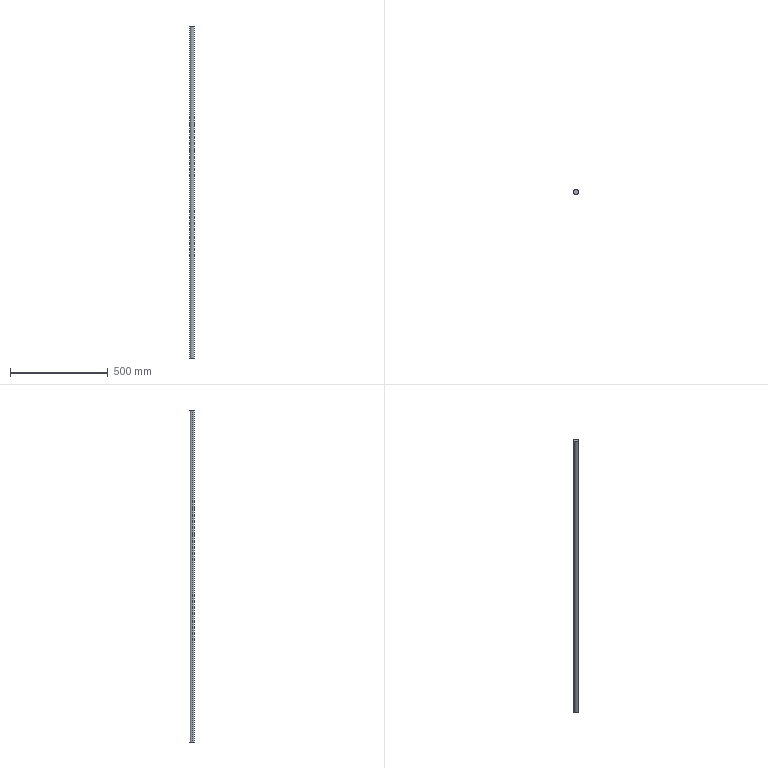Part | STEP file | 管-1700 | 1 solid | 4 faces | box 25.4 x 25.4 x 1700 mm | volume 861403 mm3 | cylinder 2 | plane 2 | commonest cylinder face diameters 25.4 x2
STEP:
#1=CARTESIAN_POINT('',(0.,0.,0.));
#2=DIRECTION('',(0.,0.,1.));
#3=DIRECTION('',(1.,0.,0.));
#4=AXIS2_PLACEMENT_3D('',#1,#2,#3);
#5=CARTESIAN_POINT('',(12.7,0.,850.));
#6=VERTEX_POINT('',#5);
#7=CARTESIAN_POINT('',(-12.7,0.,850.));
#8=VERTEX_POINT('',#7);
#9=CARTESIAN_POINT('',(0.,0.,850.));
#10=DIRECTION('',(0.,0.,1.));
#11=DIRECTION('',(1.,0.,0.));
#12=AXIS2_PLACEMENT_3D('',#9,#10,#11);
#13=CIRCLE('',#12,12.7);
#14=CARTESIAN_POINT('',(0.,0.,850.));
#15=DIRECTION('',(0.,0.,-1.));
#16=DIRECTION('',(-1.,0.,0.));
#17=AXIS2_PLACEMENT_3D('',#14,#15,#16);
#18=CYLINDRICAL_SURFACE('',#17,12.7);
#19=CARTESIAN_POINT('',(3.142,0.));
#20=DIRECTION('',(-1.,0.));
#21=VECTOR('',#20,1.);
#22=LINE('',#19,#21);
#23=(GEOMETRIC_REPRESENTATION_CONTEXT(2)PARAMETRIC_REPRESENTATION_CONTEXT()REPRESENTATION_CONTEXT('',''));
#24=DEFINITIONAL_REPRESENTATION('',(#22),#23);
#25=PCURVE('',#18,#24);
#26=CARTESIAN_POINT('',(0.,0.,850.));
#27=DIRECTION('',(0.,0.,1.));
#28=DIRECTION('',(1.,0.,0.));
#29=AXIS2_PLACEMENT_3D('',#26,#27,#28);
#30=PLANE('',#29);
#31=CARTESIAN_POINT('',(0.,0.));
#32=DIRECTION('',(1.,0.));
#33=AXIS2_PLACEMENT_2D('',#31,#32);
#34=CIRCLE('',#33,12.7);
#35=(GEOMETRIC_REPRESENTATION_CONTEXT(2)PARAMETRIC_REPRESENTATION_CONTEXT()REPRESENTATION_CONTEXT('',''));
#36=DEFINITIONAL_REPRESENTATION('',(#34),#35);
#37=PCURVE('',#30,#36);
#38=SURFACE_CURVE('',#13,(#25,#37),.PCURVE_S1.);
#39=EDGE_CURVE('',#6,#8,#38,.T.);
#40=ORIENTED_EDGE('',*,*,#39,.F.);
#41=CARTESIAN_POINT('',(12.7,0.,-850.));
#42=VERTEX_POINT('',#41);
#43=CARTESIAN_POINT('',(12.7,0.,850.));
#44=DIRECTION('',(0.,0.,-1.));
#45=VECTOR('',#44,1.);
#46=LINE('',#43,#45);
#47=CARTESIAN_POINT('',(3.142,0.));
#48=DIRECTION('',(0.,1.));
#49=VECTOR('',#48,1.);
#50=LINE('',#47,#49);
#51=(GEOMETRIC_REPRESENTATION_CONTEXT(2)PARAMETRIC_REPRESENTATION_CONTEXT()REPRESENTATION_CONTEXT('',''));
#52=DEFINITIONAL_REPRESENTATION('',(#50),#51);
#53=PCURVE('',#18,#52);
#54=CARTESIAN_POINT('',(0.,0.,850.));
#55=DIRECTION('',(0.,0.,-1.));
#56=DIRECTION('',(-1.,0.,0.));
#57=AXIS2_PLACEMENT_3D('',#54,#55,#56);
#58=CYLINDRICAL_SURFACE('',#57,12.7);
#59=CARTESIAN_POINT('',(3.142,0.));
#60=DIRECTION('',(0.,1.));
#61=VECTOR('',#60,1.);
#62=LINE('',#59,#61);
#63=(GEOMETRIC_REPRESENTATION_CONTEXT(2)PARAMETRIC_REPRESENTATION_CONTEXT()REPRESENTATION_CONTEXT('',''));
#64=DEFINITIONAL_REPRESENTATION('',(#62),#63);
#65=PCURVE('',#58,#64);
#66=SURFACE_CURVE('',#46,(#53,#65),.PCURVE_S1.);
#67=EDGE_CURVE('',#6,#42,#66,.T.);
#68=ORIENTED_EDGE('',*,*,#67,.T.);
#69=CARTESIAN_POINT('',(-12.7,0.,-850.));
#70=VERTEX_POINT('',#69);
#71=CARTESIAN_POINT('',(0.,0.,-850.));
#72=DIRECTION('',(0.,0.,1.));
#73=DIRECTION('',(1.,0.,0.));
#74=AXIS2_PLACEMENT_3D('',#71,#72,#73);
#75=CIRCLE('',#74,12.7);
#76=CARTESIAN_POINT('',(3.142,1700.));
#77=DIRECTION('',(-1.,0.));
#78=VECTOR('',#77,1.);
#79=LINE('',#76,#78);
#80=(GEOMETRIC_REPRESENTATION_CONTEXT(2)PARAMETRIC_REPRESENTATION_CONTEXT()REPRESENTATION_CONTEXT('',''));
#81=DEFINITIONAL_REPRESENTATION('',(#79),#80);
#82=PCURVE('',#18,#81);
#83=CARTESIAN_POINT('',(0.,0.,-850.));
#84=DIRECTION('',(0.,0.,1.));
#85=DIRECTION('',(1.,0.,0.));
#86=AXIS2_PLACEMENT_3D('',#83,#84,#85);
#87=PLANE('',#86);
#88=CARTESIAN_POINT('',(0.,0.));
#89=DIRECTION('',(1.,0.));
#90=AXIS2_PLACEMENT_2D('',#88,#89);
#91=CIRCLE('',#90,12.7);
#92=(GEOMETRIC_REPRESENTATION_CONTEXT(2)PARAMETRIC_REPRESENTATION_CONTEXT()REPRESENTATION_CONTEXT('',''));
#93=DEFINITIONAL_REPRESENTATION('',(#91),#92);
#94=PCURVE('',#87,#93);
#95=SURFACE_CURVE('',#75,(#82,#94),.PCURVE_S1.);
#96=EDGE_CURVE('',#42,#70,#95,.T.);
#97=ORIENTED_EDGE('',*,*,#96,.T.);
#98=CARTESIAN_POINT('',(-12.7,0.,850.));
#99=DIRECTION('',(0.,0.,-1.));
#100=VECTOR('',#99,1.);
#101=LINE('',#98,#100);
#102=CARTESIAN_POINT('',(0.,0.));
#103=DIRECTION('',(0.,1.));
#104=VECTOR('',#103,1.);
#105=LINE('',#102,#104);
#106=(GEOMETRIC_REPRESENTATION_CONTEXT(2)PARAMETRIC_REPRESENTATION_CONTEXT()REPRESENTATION_CONTEXT('',''));
#107=DEFINITIONAL_REPRESENTATION('',(#105),#106);
#108=PCURVE('',#18,#107);
#109=CARTESIAN_POINT('',(6.283,0.));
#110=DIRECTION('',(0.,1.));
#111=VECTOR('',#110,1.);
#112=LINE('',#109,#111);
#113=(GEOMETRIC_REPRESENTATION_CONTEXT(2)PARAMETRIC_REPRESENTATION_CONTEXT()REPRESENTATION_CONTEXT('',''));
#114=DEFINITIONAL_REPRESENTATION('',(#112),#113);
#115=PCURVE('',#58,#114);
#116=SURFACE_CURVE('',#101,(#108,#115),.PCURVE_S1.);
#117=EDGE_CURVE('',#8,#70,#116,.T.);
#118=ORIENTED_EDGE('',*,*,#117,.F.);
#119=EDGE_LOOP('',(#40,#68,#97,#118));
#120=FACE_BOUND('',#119,.T.);
#121=ADVANCED_FACE('',(#120),#18,.T.);
#122=ORIENTED_EDGE('',*,*,#67,.F.);
#123=CARTESIAN_POINT('',(0.,0.,850.));
#124=DIRECTION('',(0.,0.,1.));
#125=DIRECTION('',(1.,0.,0.));
#126=AXIS2_PLACEMENT_3D('',#123,#124,#125);
#127=CIRCLE('',#126,12.7);
#128=CARTESIAN_POINT('',(9.425,0.));
#129=DIRECTION('',(-1.,0.));
#130=VECTOR('',#129,1.);
#131=LINE('',#128,#130);
#132=(GEOMETRIC_REPRESENTATION_CONTEXT(2)PARAMETRIC_REPRESENTATION_CONTEXT()REPRESENTATION_CONTEXT('',''));
#133=DEFINITIONAL_REPRESENTATION('',(#131),#132);
#134=PCURVE('',#58,#133);
#135=CARTESIAN_POINT('',(0.,0.));
#136=DIRECTION('',(1.,0.));
#137=AXIS2_PLACEMENT_2D('',#135,#136);
#138=CIRCLE('',#137,12.7);
#139=(GEOMETRIC_REPRESENTATION_CONTEXT(2)PARAMETRIC_REPRESENTATION_CONTEXT()REPRESENTATION_CONTEXT('',''));
#140=DEFINITIONAL_REPRESENTATION('',(#138),#139);
#141=PCURVE('',#30,#140);
#142=SURFACE_CURVE('',#127,(#134,#141),.PCURVE_S1.);
#143=EDGE_CURVE('',#8,#6,#142,.T.);
#144=ORIENTED_EDGE('',*,*,#143,.F.);
#145=ORIENTED_EDGE('',*,*,#117,.T.);
#146=CARTESIAN_POINT('',(0.,0.,-850.));
#147=DIRECTION('',(0.,0.,1.));
#148=DIRECTION('',(1.,0.,0.));
#149=AXIS2_PLACEMENT_3D('',#146,#147,#148);
#150=CIRCLE('',#149,12.7);
#151=CARTESIAN_POINT('',(9.425,1700.));
#152=DIRECTION('',(-1.,0.));
#153=VECTOR('',#152,1.);
#154=LINE('',#151,#153);
#155=(GEOMETRIC_REPRESENTATION_CONTEXT(2)PARAMETRIC_REPRESENTATION_CONTEXT()REPRESENTATION_CONTEXT('',''));
#156=DEFINITIONAL_REPRESENTATION('',(#154),#155);
#157=PCURVE('',#58,#156);
#158=CARTESIAN_POINT('',(0.,0.));
#159=DIRECTION('',(1.,0.));
#160=AXIS2_PLACEMENT_2D('',#158,#159);
#161=CIRCLE('',#160,12.7);
#162=(GEOMETRIC_REPRESENTATION_CONTEXT(2)PARAMETRIC_REPRESENTATION_CONTEXT()REPRESENTATION_CONTEXT('',''));
#163=DEFINITIONAL_REPRESENTATION('',(#161),#162);
#164=PCURVE('',#87,#163);
#165=SURFACE_CURVE('',#150,(#157,#164),.PCURVE_S1.);
#166=EDGE_CURVE('',#70,#42,#165,.T.);
#167=ORIENTED_EDGE('',*,*,#166,.T.);
#168=EDGE_LOOP('',(#122,#144,#145,#167));
#169=FACE_BOUND('',#168,.T.);
#170=ADVANCED_FACE('',(#169),#58,.T.);
#171=ORIENTED_EDGE('',*,*,#143,.T.);
#172=ORIENTED_EDGE('',*,*,#39,.T.);
#173=EDGE_LOOP('',(#171,#172));
#174=FACE_BOUND('',#173,.T.);
#175=ADVANCED_FACE('',(#174),#30,.T.);
#176=ORIENTED_EDGE('',*,*,#166,.F.);
#177=ORIENTED_EDGE('',*,*,#96,.F.);
#178=EDGE_LOOP('',(#176,#177));
#179=FACE_BOUND('',#178,.T.);
#180=ADVANCED_FACE('',(#179),#87,.F.);
#181=CLOSED_SHELL('',(#121,#170,#175,#180));
#182=MANIFOLD_SOLID_BREP('',#181);
#183=(LENGTH_UNIT()NAMED_UNIT(*)SI_UNIT(.MILLI.,.METRE.));
#184=UNCERTAINTY_MEASURE_WITH_UNIT(LENGTH_MEASURE(0.0000001),#183,'','');
#185=(NAMED_UNIT(*)PLANE_ANGLE_UNIT()SI_UNIT($,.RADIAN.));
#186=(NAMED_UNIT(*)SI_UNIT($,.STERADIAN.)SOLID_ANGLE_UNIT());
#187=(GEOMETRIC_REPRESENTATION_CONTEXT(3)GLOBAL_UNCERTAINTY_ASSIGNED_CONTEXT((#184))GLOBAL_UNIT_ASSIGNED_CONTEXT((#183,#185,#186))REPRESENTATION_CONTEXT('',''));
#188=ADVANCED_BREP_SHAPE_REPRESENTATION('',(#4,#182),#187);